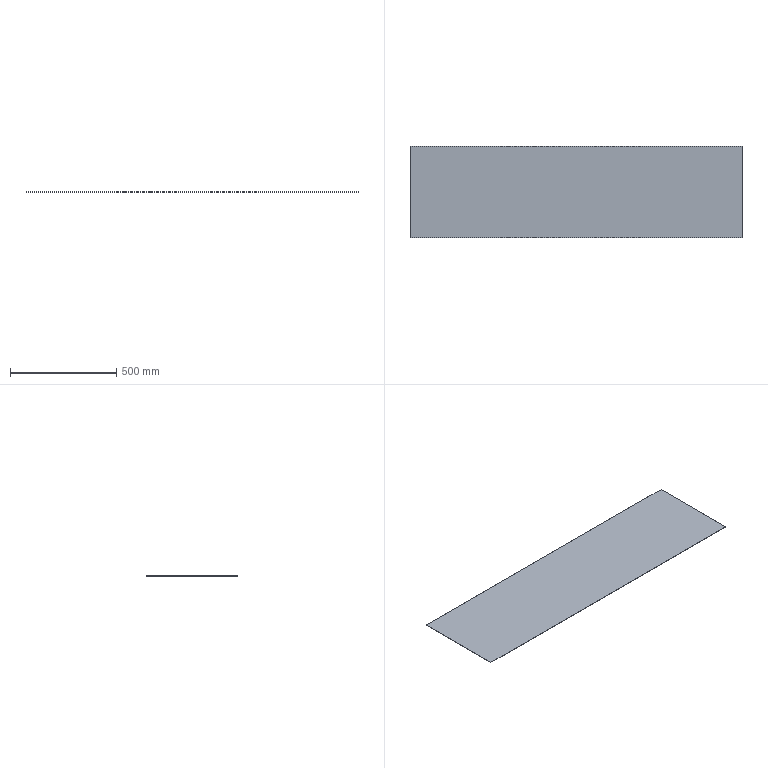Part | SolidWorks | features Extrusion 1 | 1 solid | 6 faces | box 1560 x 430 x 1.5 mm | volume 1006200 mm3 | plane 6
STEP:
#1=CARTESIAN_POINT('',(0.,430.,0.));
#2=VERTEX_POINT('',#1);
#3=CARTESIAN_POINT('',(0.,0.,0.));
#4=VERTEX_POINT('',#3);
#5=CARTESIAN_POINT('',(0.,0.,0.));
#6=DIRECTION('',(0.,-1.,0.));
#7=VECTOR('',#6,1000.);
#8=LINE('',#5,#7);
#9=EDGE_CURVE('',#2,#4,#8,.T.);
#10=ORIENTED_EDGE('',*,*,#9,.T.);
#11=CARTESIAN_POINT('',(0.,0.,1.5));
#12=VERTEX_POINT('',#11);
#13=CARTESIAN_POINT('',(0.,0.,1.5));
#14=DIRECTION('',(0.,0.,-1.));
#15=VECTOR('',#14,1000.);
#16=LINE('',#13,#15);
#17=EDGE_CURVE('',#12,#4,#16,.T.);
#18=ORIENTED_EDGE('',*,*,#17,.F.);
#19=CARTESIAN_POINT('',(0.,430.,1.5));
#20=VERTEX_POINT('',#19);
#21=CARTESIAN_POINT('',(0.,0.,1.5));
#22=DIRECTION('',(0.,-1.,0.));
#23=VECTOR('',#22,1000.);
#24=LINE('',#21,#23);
#25=EDGE_CURVE('',#20,#12,#24,.T.);
#26=ORIENTED_EDGE('',*,*,#25,.F.);
#27=CARTESIAN_POINT('',(0.,430.,1.5));
#28=DIRECTION('',(0.,0.,-1.));
#29=VECTOR('',#28,1000.);
#30=LINE('',#27,#29);
#31=EDGE_CURVE('',#20,#2,#30,.T.);
#32=ORIENTED_EDGE('',*,*,#31,.T.);
#33=EDGE_LOOP('',(#10,#18,#26,#32));
#34=FACE_OUTER_BOUND('',#33,.T.);
#35=CARTESIAN_POINT('',(0.,0.,1.5));
#36=DIRECTION('',(1.,0.,0.));
#37=DIRECTION('',(0.,0.,-1.));
#38=AXIS2_PLACEMENT_3D('',#35,#36,#37);
#39=PLANE('',#38);
#40=ADVANCED_FACE('',(#34),#39,.F.);
#41=CARTESIAN_POINT('',(1560.,0.,0.));
#42=VERTEX_POINT('',#41);
#43=CARTESIAN_POINT('',(0.,0.,0.));
#44=DIRECTION('',(1.,0.,0.));
#45=VECTOR('',#44,1000.);
#46=LINE('',#43,#45);
#47=EDGE_CURVE('',#4,#42,#46,.T.);
#48=ORIENTED_EDGE('',*,*,#47,.T.);
#49=CARTESIAN_POINT('',(1560.,0.,1.5));
#50=VERTEX_POINT('',#49);
#51=CARTESIAN_POINT('',(1560.,0.,1.5));
#52=DIRECTION('',(0.,0.,-1.));
#53=VECTOR('',#52,1000.);
#54=LINE('',#51,#53);
#55=EDGE_CURVE('',#50,#42,#54,.T.);
#56=ORIENTED_EDGE('',*,*,#55,.F.);
#57=CARTESIAN_POINT('',(0.,0.,1.5));
#58=DIRECTION('',(1.,0.,0.));
#59=VECTOR('',#58,1000.);
#60=LINE('',#57,#59);
#61=EDGE_CURVE('',#12,#50,#60,.T.);
#62=ORIENTED_EDGE('',*,*,#61,.F.);
#63=ORIENTED_EDGE('',*,*,#17,.T.);
#64=EDGE_LOOP('',(#48,#56,#62,#63));
#65=FACE_OUTER_BOUND('',#64,.T.);
#66=CARTESIAN_POINT('',(0.,0.,1.5));
#67=DIRECTION('',(0.,1.,0.));
#68=DIRECTION('',(0.,0.,1.));
#69=AXIS2_PLACEMENT_3D('',#66,#67,#68);
#70=PLANE('',#69);
#71=ADVANCED_FACE('',(#65),#70,.F.);
#72=CARTESIAN_POINT('',(1560.,430.,0.));
#73=VERTEX_POINT('',#72);
#74=CARTESIAN_POINT('',(1560.,0.,0.));
#75=DIRECTION('',(0.,1.,0.));
#76=VECTOR('',#75,1000.);
#77=LINE('',#74,#76);
#78=EDGE_CURVE('',#42,#73,#77,.T.);
#79=ORIENTED_EDGE('',*,*,#78,.T.);
#80=CARTESIAN_POINT('',(1560.,430.,1.5));
#81=VERTEX_POINT('',#80);
#82=CARTESIAN_POINT('',(1560.,430.,1.5));
#83=DIRECTION('',(0.,0.,-1.));
#84=VECTOR('',#83,1000.);
#85=LINE('',#82,#84);
#86=EDGE_CURVE('',#81,#73,#85,.T.);
#87=ORIENTED_EDGE('',*,*,#86,.F.);
#88=CARTESIAN_POINT('',(1560.,0.,1.5));
#89=DIRECTION('',(0.,1.,0.));
#90=VECTOR('',#89,1000.);
#91=LINE('',#88,#90);
#92=EDGE_CURVE('',#50,#81,#91,.T.);
#93=ORIENTED_EDGE('',*,*,#92,.F.);
#94=ORIENTED_EDGE('',*,*,#55,.T.);
#95=EDGE_LOOP('',(#79,#87,#93,#94));
#96=FACE_OUTER_BOUND('',#95,.T.);
#97=CARTESIAN_POINT('',(1560.,0.,1.5));
#98=DIRECTION('',(-1.,0.,0.));
#99=DIRECTION('',(0.,0.,1.));
#100=AXIS2_PLACEMENT_3D('',#97,#98,#99);
#101=PLANE('',#100);
#102=ADVANCED_FACE('',(#96),#101,.F.);
#103=CARTESIAN_POINT('',(0.,430.,0.));
#104=DIRECTION('',(-1.,0.,0.));
#105=VECTOR('',#104,1000.);
#106=LINE('',#103,#105);
#107=EDGE_CURVE('',#73,#2,#106,.T.);
#108=ORIENTED_EDGE('',*,*,#107,.T.);
#109=ORIENTED_EDGE('',*,*,#31,.F.);
#110=CARTESIAN_POINT('',(0.,430.,1.5));
#111=DIRECTION('',(-1.,0.,0.));
#112=VECTOR('',#111,1000.);
#113=LINE('',#110,#112);
#114=EDGE_CURVE('',#81,#20,#113,.T.);
#115=ORIENTED_EDGE('',*,*,#114,.F.);
#116=ORIENTED_EDGE('',*,*,#86,.T.);
#117=EDGE_LOOP('',(#108,#109,#115,#116));
#118=FACE_OUTER_BOUND('',#117,.T.);
#119=CARTESIAN_POINT('',(0.,430.,1.5));
#120=DIRECTION('',(0.,-1.,0.));
#121=DIRECTION('',(0.,0.,-1.));
#122=AXIS2_PLACEMENT_3D('',#119,#120,#121);
#123=PLANE('',#122);
#124=ADVANCED_FACE('',(#118),#123,.F.);
#125=ORIENTED_EDGE('',*,*,#25,.T.);
#126=ORIENTED_EDGE('',*,*,#61,.T.);
#127=ORIENTED_EDGE('',*,*,#92,.T.);
#128=ORIENTED_EDGE('',*,*,#114,.T.);
#129=EDGE_LOOP('',(#125,#126,#127,#128));
#130=FACE_OUTER_BOUND('',#129,.T.);
#131=CARTESIAN_POINT('',(0.,0.,1.5));
#132=DIRECTION('',(0.,0.,-1.));
#133=DIRECTION('',(-1.,0.,0.));
#134=AXIS2_PLACEMENT_3D('',#131,#132,#133);
#135=PLANE('',#134);
#136=ADVANCED_FACE('',(#130),#135,.F.);
#137=ORIENTED_EDGE('',*,*,#9,.F.);
#138=ORIENTED_EDGE('',*,*,#107,.F.);
#139=ORIENTED_EDGE('',*,*,#78,.F.);
#140=ORIENTED_EDGE('',*,*,#47,.F.);
#141=EDGE_LOOP('',(#137,#138,#139,#140));
#142=FACE_OUTER_BOUND('',#141,.T.);
#143=CARTESIAN_POINT('',(0.,0.,0.));
#144=DIRECTION('',(0.,0.,-1.));
#145=DIRECTION('',(-1.,0.,0.));
#146=AXIS2_PLACEMENT_3D('',#143,#144,#145);
#147=PLANE('',#146);
#148=ADVANCED_FACE('',(#142),#147,.T.);
#149=CLOSED_SHELL('',(#40,#71,#102,#124,#136,#148));
#150=MANIFOLD_SOLID_BREP('',#149);
#151=CARTESIAN_POINT('',(0.,0.,0.));
#152=DIRECTION('',(0.,0.,1.));
#153=DIRECTION('',(1.,0.,0.));
#154=AXIS2_PLACEMENT_3D('',#151,#152,#153);
#155=(LENGTH_UNIT()NAMED_UNIT(*)SI_UNIT(.MILLI.,.METRE.));
#156=UNCERTAINTY_MEASURE_WITH_UNIT(LENGTH_MEASURE(0.00001),#155,'','');
#157=(NAMED_UNIT(*)PLANE_ANGLE_UNIT()SI_UNIT($,.RADIAN.));
#158=(NAMED_UNIT(*)SI_UNIT($,.STERADIAN.)SOLID_ANGLE_UNIT());
#159=(GEOMETRIC_REPRESENTATION_CONTEXT(3)GLOBAL_UNCERTAINTY_ASSIGNED_CONTEXT((#156))GLOBAL_UNIT_ASSIGNED_CONTEXT((#155,#157,#158))REPRESENTATION_CONTEXT('',''));
#160=ADVANCED_BREP_SHAPE_REPRESENTATION('',(#150,#154),#159);